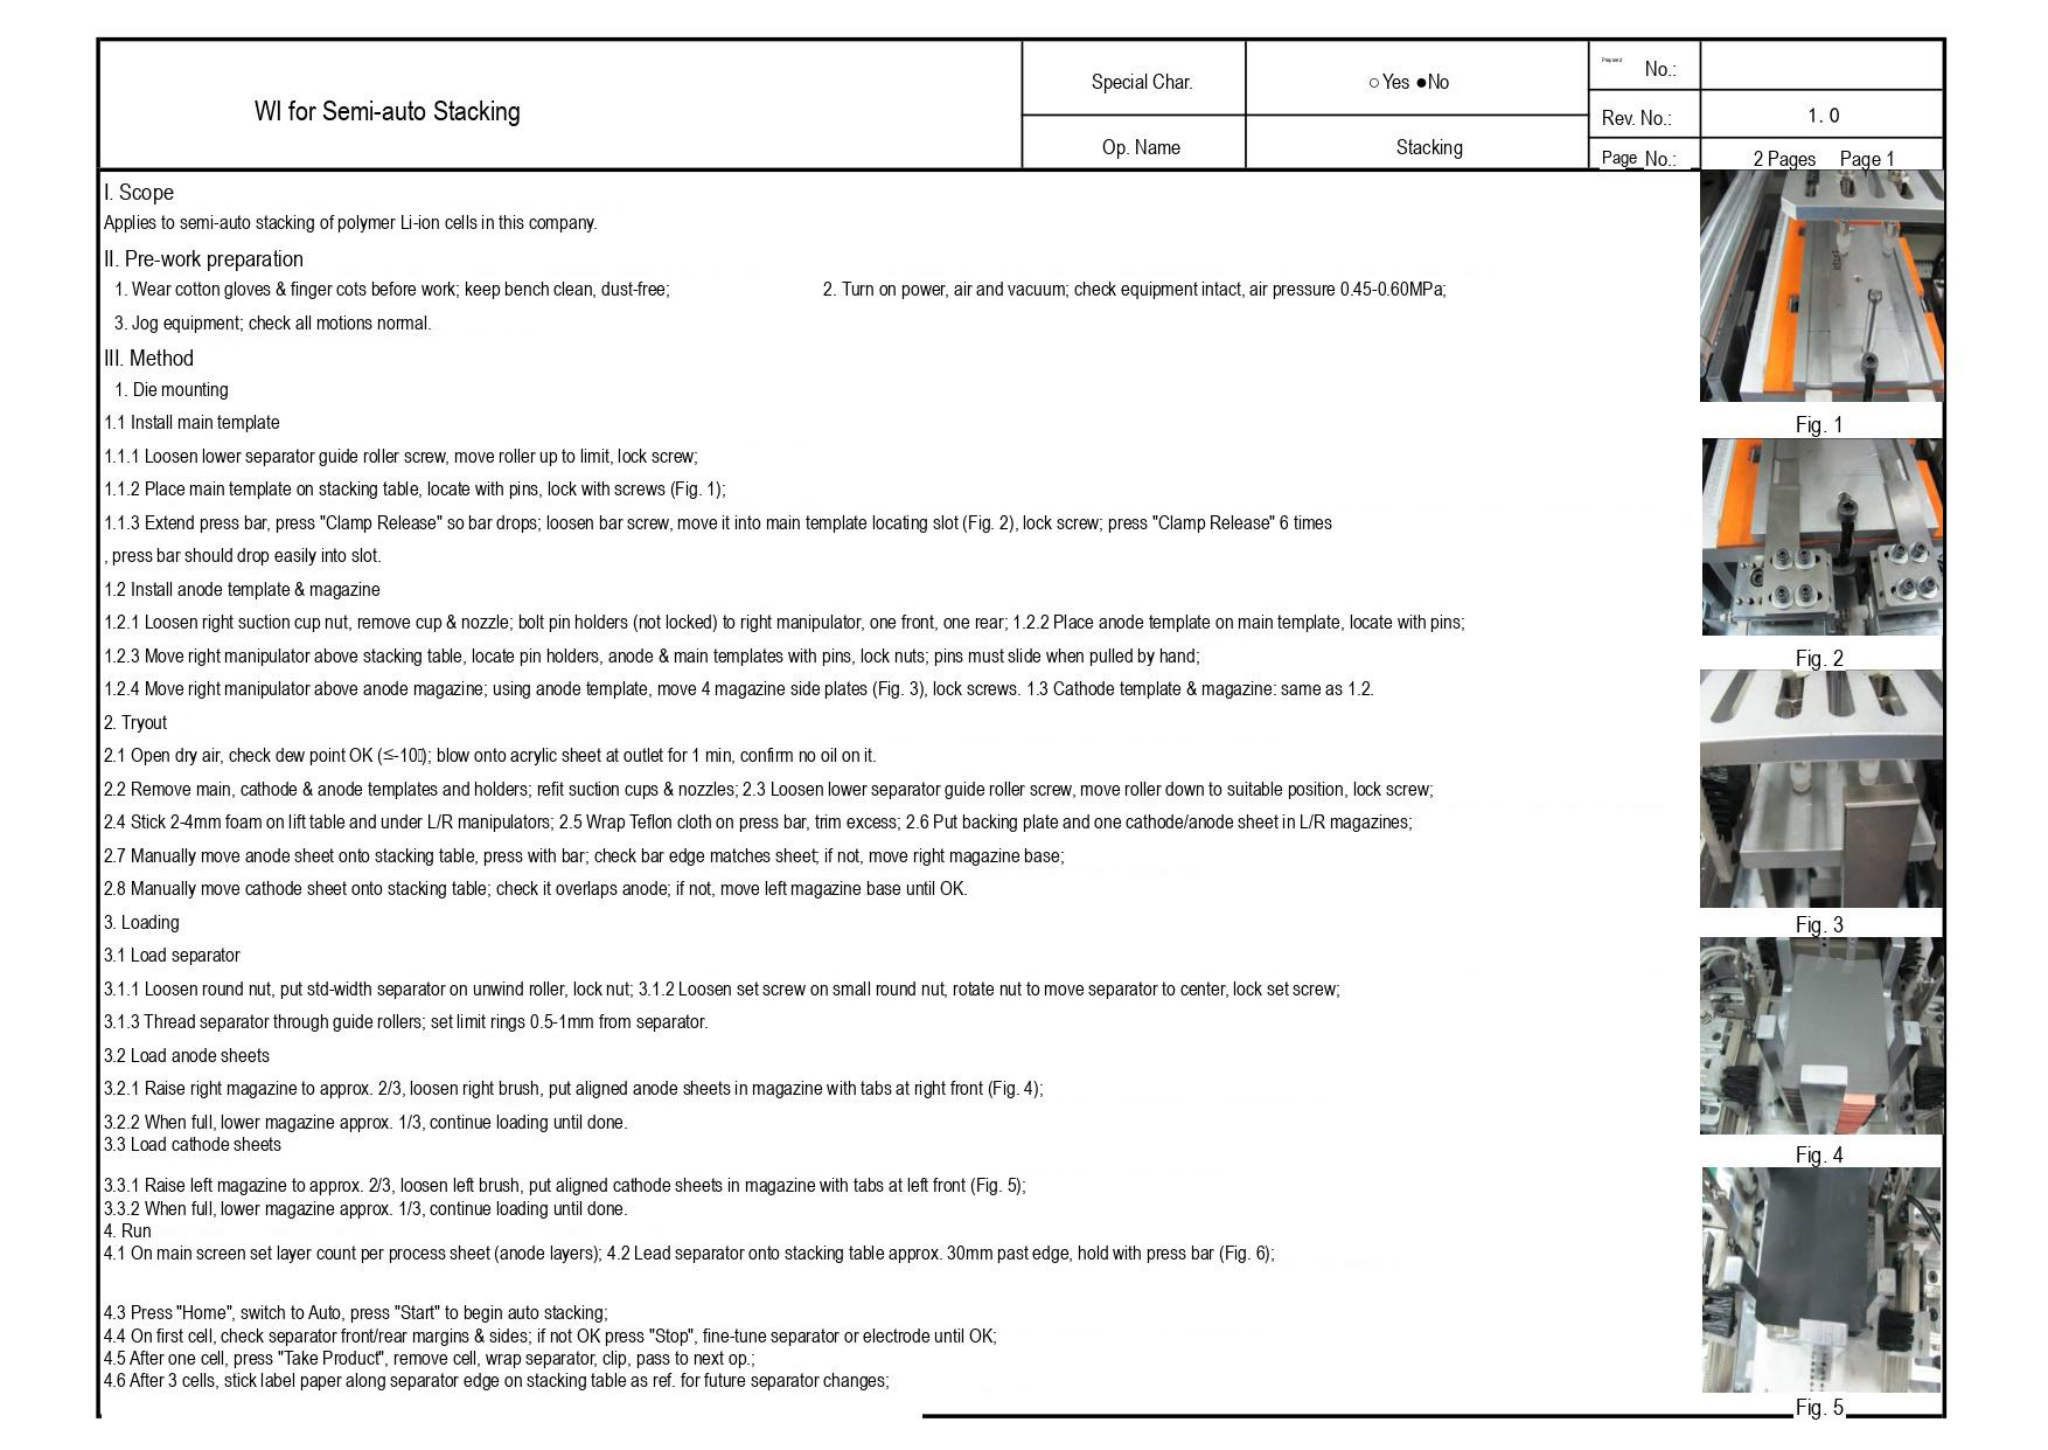| WI for Semi-auto Stacking | Special Char. | ○Yes ●No | No.: | |
|---|---|---|---|---|
| | | | Rev. No.: | 1. 0 |
| | Op. Name | Stacking | Page No.: | 2 Pages Page 1 |

I. Scope

Applies to semi-auto stacking of polymer Li-ion cells in this company.

II. Pre-work preparation

1. Wear cotton gloves & finger cots before work; keep bench clean, dust-free;

2. Turn on power, air and vacuum; check equipment intact, air pressure 0.45-0.60MPa;

3. Jog equipment; check all motions normal.

III. Method

1. Die mounting

1.1 Install main template

1.1.1 Loosen lower separator guide roller screw, move roller up to limit, lock screw;

1.1.2 Place main template on stacking table, locate with pins, lock with screws (Fig. 1);

1.1.3 Extend press bar, press "Clamp Release" so bar drops; loosen bar screw, move it into main template locating slot (Fig. 2), lock screw; press "Clamp Release" 6 times

, press bar should drop easily into slot.

1.2 Install anode template & magazine

1.2.1 Loosen right suction cup nut, remove cup & nozzle; bolt pin holders (not locked) to right manipulator, one front, one rear; 1.2.2 Place anode template on main template, locate with pins;

1.2.3 Move right manipulator above stacking table, locate pin holders, anode & main templates with pins, lock nuts; pins must slide when pulled by hand;

1.2.4 Move right manipulator above anode magazine; using anode template, move 4 magazine side plates (Fig. 3), lock screws. 1.3 Cathode template & magazine: same as 1.2.

2. Tryout

2.1 Open dry air, check dew point OK (≤-10); blow onto acrylic sheet at outlet for 1 min, confirm no oil on it.

2.2 Remove main, cathode & anode templates and holders; refit suction cups & nozzles; 2.3 Loosen lower separator guide roller screw, move roller down to suitable position, lock screw;

2.4 Stick 2-4mm foam on lift table and under L/R manipulators; 2.5 Wrap Teflon cloth on press bar, trim excess; 2.6 Put backing plate and one cathode/anode sheet in L/R magazines;

2.7 Manually move anode sheet onto stacking table, press with bar; check bar edge matches sheet; if not, move right magazine base;

2.8 Manually move cathode sheet onto stacking table; check it overlaps anode; if not, move left magazine base until OK.

3. Loading

3.1 Load separator

3.1.1 Loosen round nut, put std-width separator on unwind roller, lock nut; 3.1.2 Loosen set screw on small round nut, rotate nut to move separator to center, lock set screw;

3.1.3 Thread separator through guide rollers; set limit rings 0.5-1mm from separator.

3.2 Load anode sheets

3.2.1 Raise right magazine to approx. 2/3, loosen right brush, put aligned anode sheets in magazine with tabs at right front (Fig. 4);

3.2.2 When full, lower magazine approx. 1/3, continue loading until done.
3.3 Load cathode sheets

3.3.1 Raise left magazine to approx. 2/3, loosen left brush, put aligned cathode sheets in magazine with tabs at left front (Fig. 5);
3.3.2 When full, lower magazine approx. 1/3, continue loading until done.
4. Run
4.1 On main screen set layer count per process sheet (anode layers); 4.2 Lead separator onto stacking table approx. 30mm past edge, hold with press bar (Fig. 6);

4.3 Press "Home", switch to Auto, press "Start" to begin auto stacking;
4.4 On first cell, check separator front/rear margins & sides; if not OK press "Stop", fine-tune separator or electrode until OK;
4.5 After one cell, press "Take Product", remove cell, wrap separator, clip, pass to next op.;
4.6 After 3 cells, stick label paper along separator edge on stacking table as ref. for future separator changes;

Fig. 1

Fig. 2

Fig. 3

Fig. 4

Fig. 5
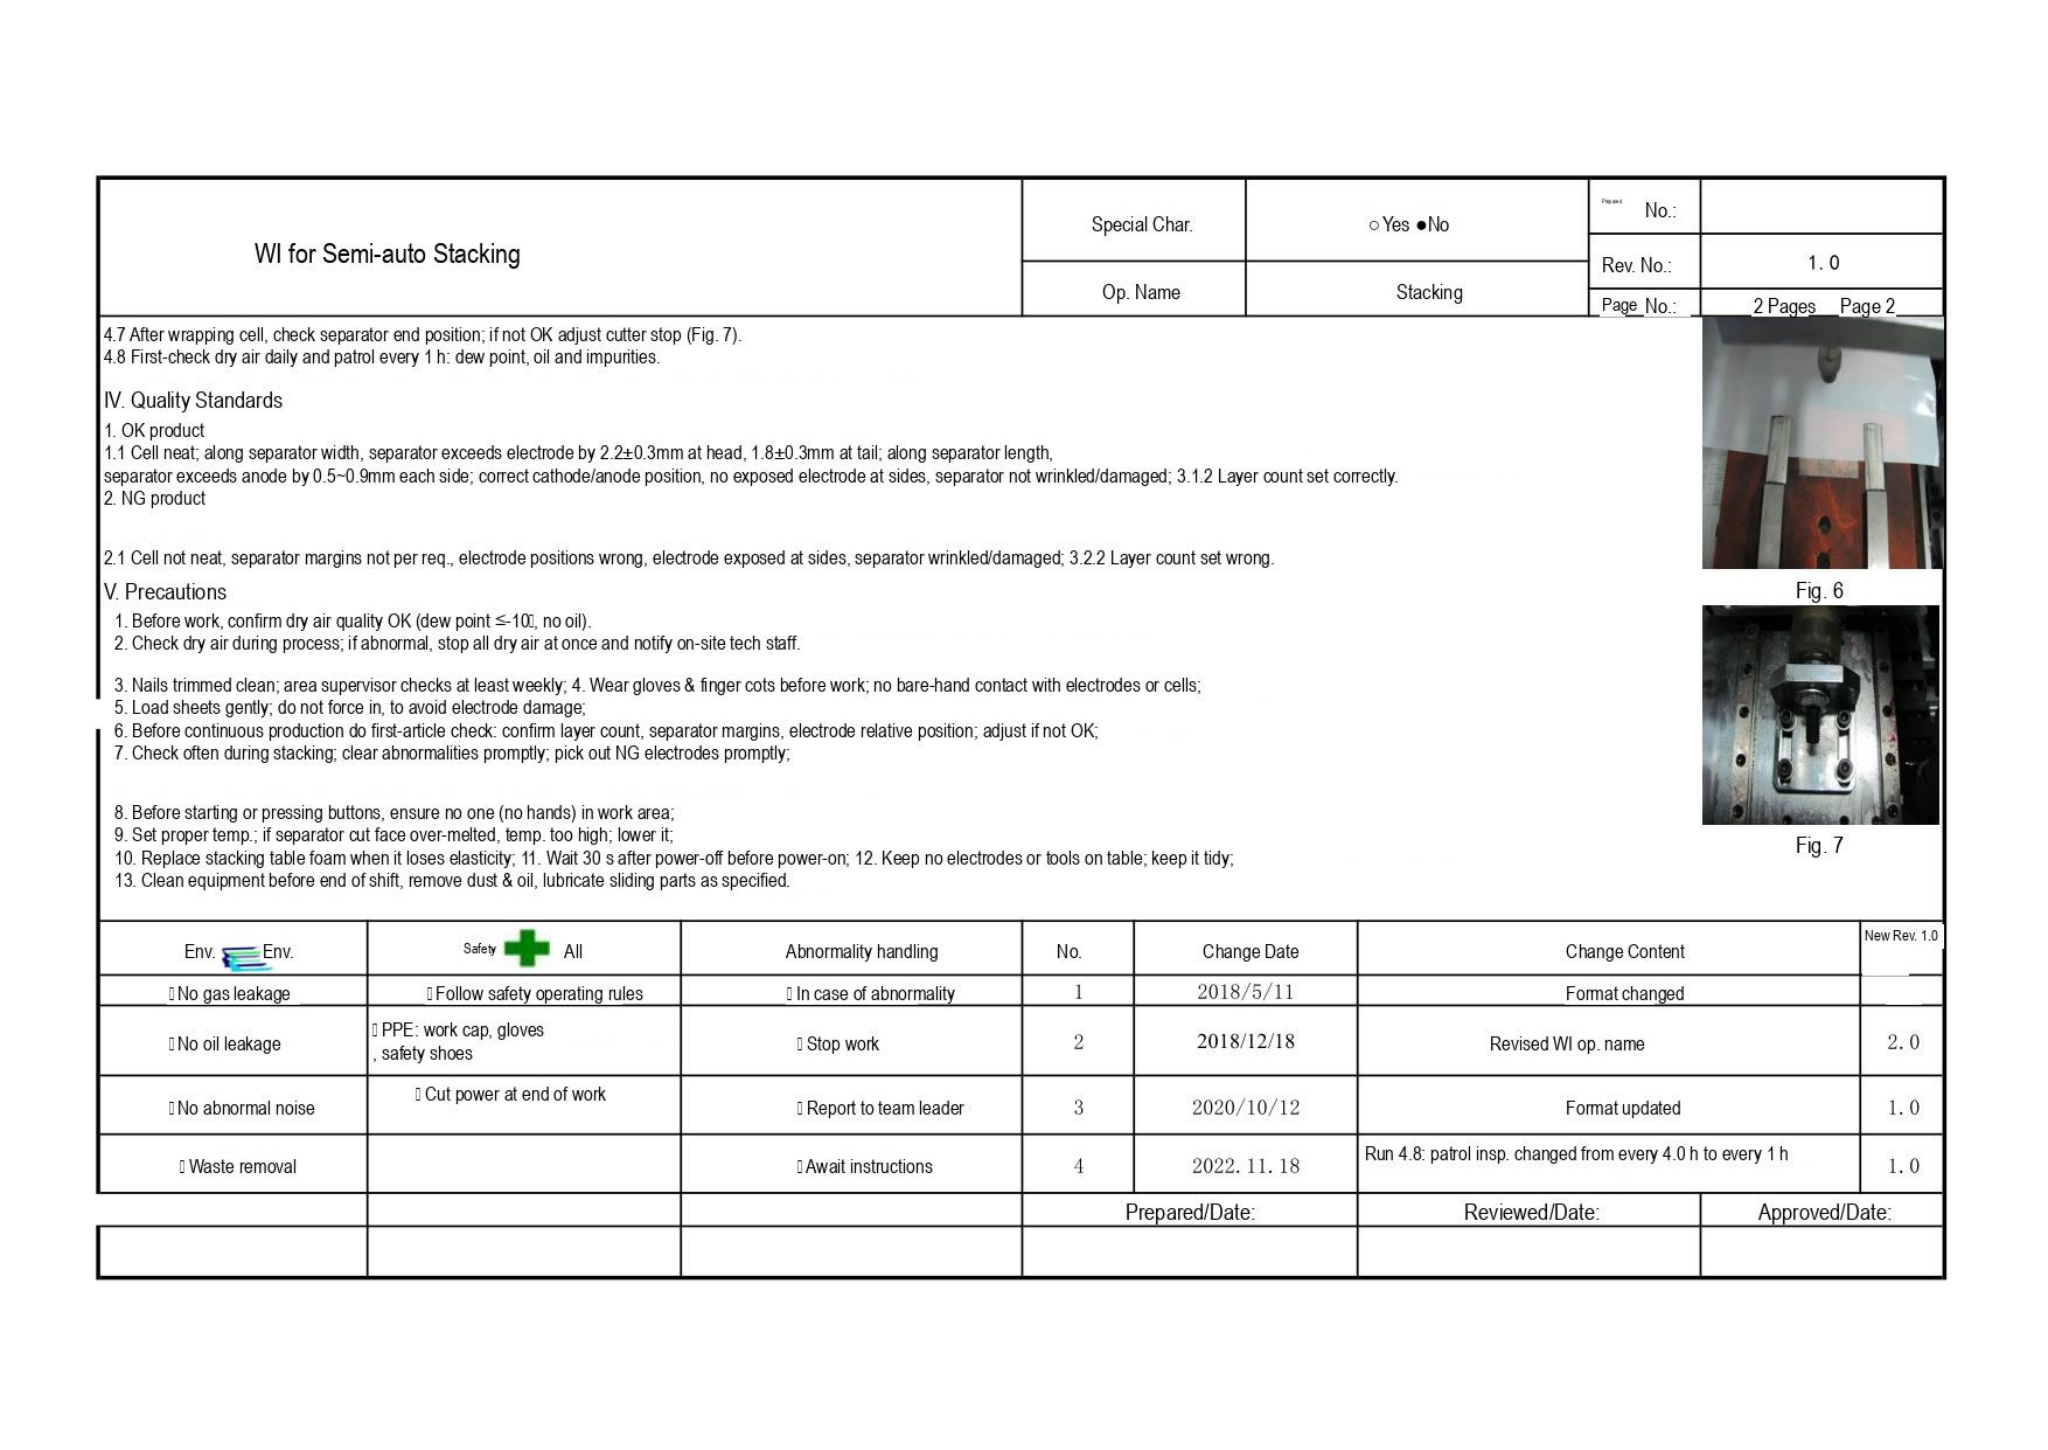| WI for Semi-auto Stacking | Special Char. | ○Yes ●No | No.: | |
|---|---|---|---|---|
| | Op. Name | Stacking | Rev. No.: | 1. 0 |
| | | | Page No.: | 2 Pages Page 2 |

4.7 After wrapping cell, check separator end position; if not OK adjust cutter stop (Fig. 7).
4.8 First-check dry air daily and patrol every 1 h: dew point, oil and impurities.

IV. Quality Standards
1. OK product
1.1 Cell neat; along separator width, separator exceeds electrode by 2.2±0.3mm at head, 1.8±0.3mm at tail; along separator length, separator exceeds anode by 0.5~0.9mm each side; correct cathode/anode position, no exposed electrode at sides, separator not wrinkled/damaged; 3.1.2 Layer count set correctly.
2. NG product

2.1 Cell not neat, separator margins not per req., electrode positions wrong, electrode exposed at sides, separator wrinkled/damaged; 3.2.2 Layer count set wrong.

V. Precautions
1. Before work, confirm dry air quality OK (dew point ≤-10, no oil).
2. Check dry air during process; if abnormal, stop all dry air at once and notify on-site tech staff.

3. Nails trimmed clean; area supervisor checks at least weekly; 4. Wear gloves & finger cots before work; no bare-hand contact with electrodes or cells;
5. Load sheets gently; do not force in, to avoid electrode damage;
6. Before continuous production do first-article check: confirm layer count, separator margins, electrode relative position; adjust if not OK;
7. Check often during stacking; clear abnormalities promptly; pick out NG electrodes promptly;

8. Before starting or pressing buttons, ensure no one (no hands) in work area;
9. Set proper temp.; if separator cut face over-melted, temp. too high; lower it;
10. Replace stacking table foam when it loses elasticity; 11. Wait 30 s after power-off before power-on; 12. Keep no electrodes or tools on table; keep it tidy;
13. Clean equipment before end of shift, remove dust & oil, lubricate sliding parts as specified.

Fig. 6

Fig. 7

| Env. Env. | Safety All | Abnormality handling | No. | Change Date | Change Content | New Rev. 1.0 |
|---|---|---|---|---|---|---|
| No gas leakage | Follow safety operating rules | In case of abnormality | 1 | 2018/5/11 | Format changed | |
| No oil leakage | PPE: work cap, gloves , safety shoes | Stop work | 2 | 2018/12/18 | Revised WI op. name | 2. 0 |
| No abnormal noise | Cut power at end of work | Report to team leader | 3 | 2020/10/12 | Format updated | 1. 0 |
| Waste removal | | Await instructions | 4 | 2022. 11. 18 | Run 4.8: patrol insp. changed from every 4.0 h to every 1 h | 1. 0 |
| | | | Prepared/Date: | | Reviewed/Date: | Approved/Date: |
| | | | | | | |